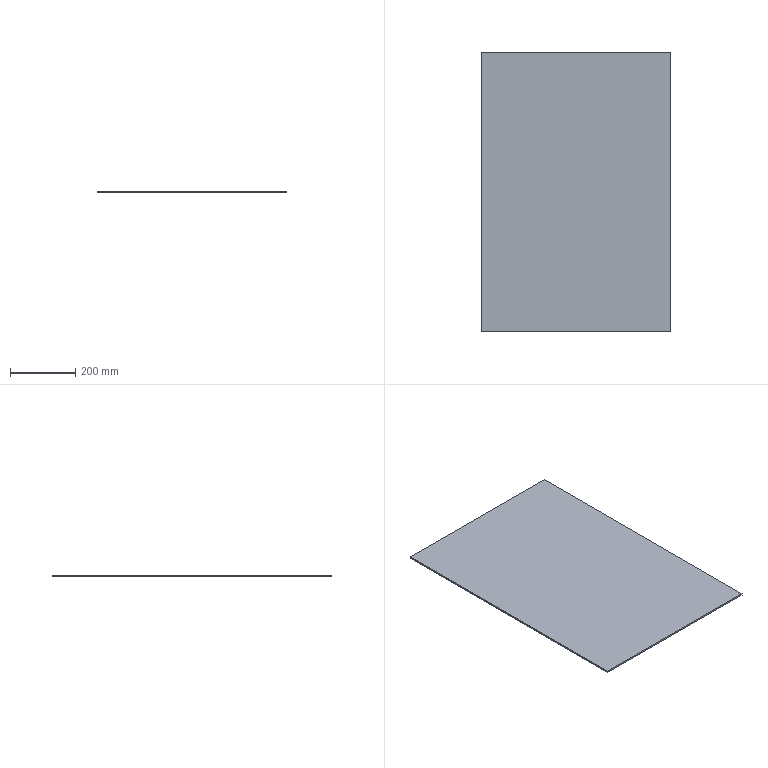Part | SolidWorks | features Extrusion 1 | 1 solid | 6 faces | box 581 x 858 x 5 mm | volume 2492490 mm3 | plane 6
STEP:
#1=CARTESIAN_POINT('',(290.5,-429.,0.));
#2=VERTEX_POINT('',#1);
#3=CARTESIAN_POINT('',(290.5,429.,0.));
#4=VERTEX_POINT('',#3);
#5=CARTESIAN_POINT('',(290.5,429.,0.));
#6=DIRECTION('',(0.,1.,0.));
#7=VECTOR('',#6,1000.);
#8=LINE('',#5,#7);
#9=EDGE_CURVE('',#2,#4,#8,.T.);
#10=ORIENTED_EDGE('',*,*,#9,.T.);
#11=CARTESIAN_POINT('',(290.5,429.,5.));
#12=VERTEX_POINT('',#11);
#13=CARTESIAN_POINT('',(290.5,429.,5.));
#14=DIRECTION('',(0.,0.,-1.));
#15=VECTOR('',#14,1000.);
#16=LINE('',#13,#15);
#17=EDGE_CURVE('',#12,#4,#16,.T.);
#18=ORIENTED_EDGE('',*,*,#17,.F.);
#19=CARTESIAN_POINT('',(290.5,-429.,5.));
#20=VERTEX_POINT('',#19);
#21=CARTESIAN_POINT('',(290.5,429.,5.));
#22=DIRECTION('',(0.,1.,0.));
#23=VECTOR('',#22,1000.);
#24=LINE('',#21,#23);
#25=EDGE_CURVE('',#20,#12,#24,.T.);
#26=ORIENTED_EDGE('',*,*,#25,.F.);
#27=CARTESIAN_POINT('',(290.5,-429.,5.));
#28=DIRECTION('',(0.,0.,-1.));
#29=VECTOR('',#28,1000.);
#30=LINE('',#27,#29);
#31=EDGE_CURVE('',#20,#2,#30,.T.);
#32=ORIENTED_EDGE('',*,*,#31,.T.);
#33=EDGE_LOOP('',(#10,#18,#26,#32));
#34=FACE_OUTER_BOUND('',#33,.T.);
#35=CARTESIAN_POINT('',(290.5,429.,5.));
#36=DIRECTION('',(-1.,0.,0.));
#37=DIRECTION('',(0.,-1.,0.));
#38=AXIS2_PLACEMENT_3D('',#35,#36,#37);
#39=PLANE('',#38);
#40=ADVANCED_FACE('',(#34),#39,.F.);
#41=CARTESIAN_POINT('',(-290.5,429.,0.));
#42=VERTEX_POINT('',#41);
#43=CARTESIAN_POINT('',(-290.5,429.,0.));
#44=DIRECTION('',(-1.,0.,0.));
#45=VECTOR('',#44,1000.);
#46=LINE('',#43,#45);
#47=EDGE_CURVE('',#4,#42,#46,.T.);
#48=ORIENTED_EDGE('',*,*,#47,.T.);
#49=CARTESIAN_POINT('',(-290.5,429.,5.));
#50=VERTEX_POINT('',#49);
#51=CARTESIAN_POINT('',(-290.5,429.,5.));
#52=DIRECTION('',(0.,0.,-1.));
#53=VECTOR('',#52,1000.);
#54=LINE('',#51,#53);
#55=EDGE_CURVE('',#50,#42,#54,.T.);
#56=ORIENTED_EDGE('',*,*,#55,.F.);
#57=CARTESIAN_POINT('',(-290.5,429.,5.));
#58=DIRECTION('',(-1.,0.,0.));
#59=VECTOR('',#58,1000.);
#60=LINE('',#57,#59);
#61=EDGE_CURVE('',#12,#50,#60,.T.);
#62=ORIENTED_EDGE('',*,*,#61,.F.);
#63=ORIENTED_EDGE('',*,*,#17,.T.);
#64=EDGE_LOOP('',(#48,#56,#62,#63));
#65=FACE_OUTER_BOUND('',#64,.T.);
#66=CARTESIAN_POINT('',(-290.5,429.,5.));
#67=DIRECTION('',(0.,-1.,0.));
#68=DIRECTION('',(0.,0.,-1.));
#69=AXIS2_PLACEMENT_3D('',#66,#67,#68);
#70=PLANE('',#69);
#71=ADVANCED_FACE('',(#65),#70,.F.);
#72=CARTESIAN_POINT('',(-290.5,-429.,0.));
#73=VERTEX_POINT('',#72);
#74=CARTESIAN_POINT('',(-290.5,429.,0.));
#75=DIRECTION('',(0.,-1.,0.));
#76=VECTOR('',#75,1000.);
#77=LINE('',#74,#76);
#78=EDGE_CURVE('',#42,#73,#77,.T.);
#79=ORIENTED_EDGE('',*,*,#78,.T.);
#80=CARTESIAN_POINT('',(-290.5,-429.,5.));
#81=VERTEX_POINT('',#80);
#82=CARTESIAN_POINT('',(-290.5,-429.,5.));
#83=DIRECTION('',(0.,0.,-1.));
#84=VECTOR('',#83,1000.);
#85=LINE('',#82,#84);
#86=EDGE_CURVE('',#81,#73,#85,.T.);
#87=ORIENTED_EDGE('',*,*,#86,.F.);
#88=CARTESIAN_POINT('',(-290.5,429.,5.));
#89=DIRECTION('',(0.,-1.,0.));
#90=VECTOR('',#89,1000.);
#91=LINE('',#88,#90);
#92=EDGE_CURVE('',#50,#81,#91,.T.);
#93=ORIENTED_EDGE('',*,*,#92,.F.);
#94=ORIENTED_EDGE('',*,*,#55,.T.);
#95=EDGE_LOOP('',(#79,#87,#93,#94));
#96=FACE_OUTER_BOUND('',#95,.T.);
#97=CARTESIAN_POINT('',(-290.5,429.,5.));
#98=DIRECTION('',(1.,0.,0.));
#99=DIRECTION('',(0.,1.,0.));
#100=AXIS2_PLACEMENT_3D('',#97,#98,#99);
#101=PLANE('',#100);
#102=ADVANCED_FACE('',(#96),#101,.F.);
#103=CARTESIAN_POINT('',(-290.5,-429.,0.));
#104=DIRECTION('',(1.,0.,0.));
#105=VECTOR('',#104,1000.);
#106=LINE('',#103,#105);
#107=EDGE_CURVE('',#73,#2,#106,.T.);
#108=ORIENTED_EDGE('',*,*,#107,.T.);
#109=ORIENTED_EDGE('',*,*,#31,.F.);
#110=CARTESIAN_POINT('',(-290.5,-429.,5.));
#111=DIRECTION('',(1.,0.,0.));
#112=VECTOR('',#111,1000.);
#113=LINE('',#110,#112);
#114=EDGE_CURVE('',#81,#20,#113,.T.);
#115=ORIENTED_EDGE('',*,*,#114,.F.);
#116=ORIENTED_EDGE('',*,*,#86,.T.);
#117=EDGE_LOOP('',(#108,#109,#115,#116));
#118=FACE_OUTER_BOUND('',#117,.T.);
#119=CARTESIAN_POINT('',(-290.5,-429.,5.));
#120=DIRECTION('',(0.,1.,0.));
#121=DIRECTION('',(0.,0.,1.));
#122=AXIS2_PLACEMENT_3D('',#119,#120,#121);
#123=PLANE('',#122);
#124=ADVANCED_FACE('',(#118),#123,.F.);
#125=ORIENTED_EDGE('',*,*,#25,.T.);
#126=ORIENTED_EDGE('',*,*,#61,.T.);
#127=ORIENTED_EDGE('',*,*,#92,.T.);
#128=ORIENTED_EDGE('',*,*,#114,.T.);
#129=EDGE_LOOP('',(#125,#126,#127,#128));
#130=FACE_OUTER_BOUND('',#129,.T.);
#131=CARTESIAN_POINT('',(0.,0.,5.));
#132=DIRECTION('',(0.,0.,1.));
#133=DIRECTION('',(1.,0.,0.));
#134=AXIS2_PLACEMENT_3D('',#131,#132,#133);
#135=PLANE('',#134);
#136=ADVANCED_FACE('',(#130),#135,.T.);
#137=ORIENTED_EDGE('',*,*,#9,.F.);
#138=ORIENTED_EDGE('',*,*,#107,.F.);
#139=ORIENTED_EDGE('',*,*,#78,.F.);
#140=ORIENTED_EDGE('',*,*,#47,.F.);
#141=EDGE_LOOP('',(#137,#138,#139,#140));
#142=FACE_OUTER_BOUND('',#141,.T.);
#143=CARTESIAN_POINT('',(0.,0.,0.));
#144=DIRECTION('',(0.,0.,1.));
#145=DIRECTION('',(1.,0.,0.));
#146=AXIS2_PLACEMENT_3D('',#143,#144,#145);
#147=PLANE('',#146);
#148=ADVANCED_FACE('',(#142),#147,.F.);
#149=CLOSED_SHELL('',(#40,#71,#102,#124,#136,#148));
#150=MANIFOLD_SOLID_BREP('',#149);
#151=CARTESIAN_POINT('',(0.,0.,0.));
#152=DIRECTION('',(0.,0.,1.));
#153=DIRECTION('',(1.,0.,0.));
#154=AXIS2_PLACEMENT_3D('',#151,#152,#153);
#155=(LENGTH_UNIT()NAMED_UNIT(*)SI_UNIT(.MILLI.,.METRE.));
#156=UNCERTAINTY_MEASURE_WITH_UNIT(LENGTH_MEASURE(0.00001),#155,'','');
#157=(NAMED_UNIT(*)PLANE_ANGLE_UNIT()SI_UNIT($,.RADIAN.));
#158=(NAMED_UNIT(*)SI_UNIT($,.STERADIAN.)SOLID_ANGLE_UNIT());
#159=(GEOMETRIC_REPRESENTATION_CONTEXT(3)GLOBAL_UNCERTAINTY_ASSIGNED_CONTEXT((#156))GLOBAL_UNIT_ASSIGNED_CONTEXT((#155,#157,#158))REPRESENTATION_CONTEXT('',''));
#160=ADVANCED_BREP_SHAPE_REPRESENTATION('',(#150,#154),#159);